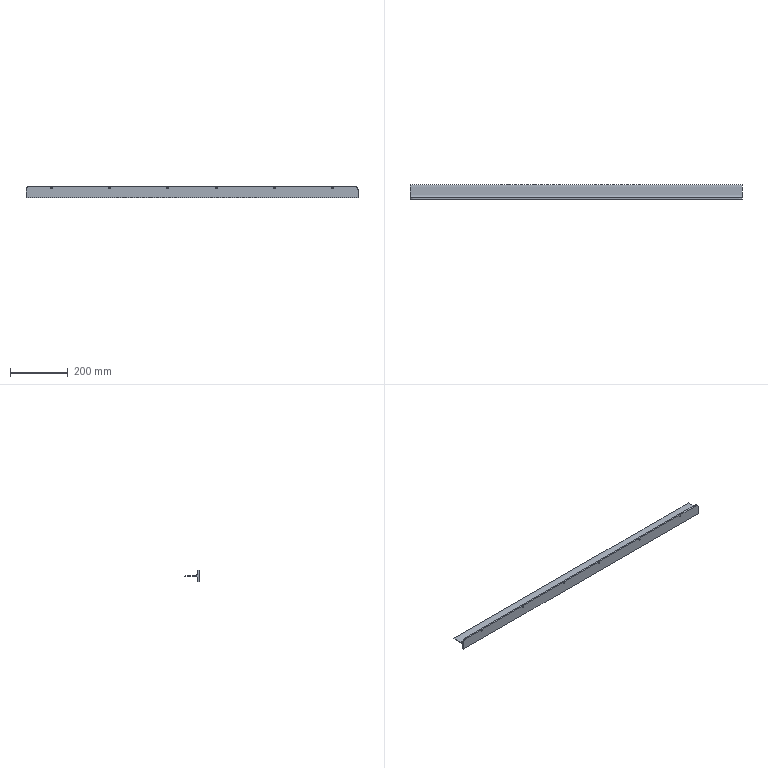Part | NX | features BREP 1 | 1 solid | 25 faces | box 1146 x 50 x 39 mm | volume 357645 mm3 | cylinder 16 | plane 7 | spline 2 | commonest cylinder face diameters 5 x12 20 x2 24 x2
STEP:
#1=CARTESIAN_POINT('',(1058.,-1.616,17.));
#2=VERTEX_POINT('',#1);
#3=CARTESIAN_POINT('',(1058.,-1.616,12.));
#4=VERTEX_POINT('',#3);
#5=CARTESIAN_POINT('',(1058.,-1.616,14.5));
#6=DIRECTION('',(0.,-1.,0.));
#7=DIRECTION('',(0.,0.,1.));
#8=AXIS2_PLACEMENT_3D('',#5,#6,#7);
#9=CIRCLE('',#8,2.5);
#10=EDGE_CURVE('',#2,#4,#9,.T.);
#11=ORIENTED_EDGE('',*,*,#10,.T.);
#12=CARTESIAN_POINT('',(1058.,3.384,12.));
#13=VERTEX_POINT('',#12);
#14=CARTESIAN_POINT('',(1058.,-1.617,12.));
#15=DIRECTION('',(0.,1.,0.));
#16=VECTOR('',#15,1000.);
#17=LINE('',#14,#16);
#18=EDGE_CURVE('',#4,#13,#17,.T.);
#19=ORIENTED_EDGE('',*,*,#18,.T.);
#20=CARTESIAN_POINT('',(1058.,3.384,17.));
#21=VERTEX_POINT('',#20);
#22=CARTESIAN_POINT('',(1058.,3.384,14.5));
#23=DIRECTION('',(0.,1.,0.));
#24=DIRECTION('',(0.,0.,-1.));
#25=AXIS2_PLACEMENT_3D('',#22,#23,#24);
#26=CIRCLE('',#25,2.5);
#27=EDGE_CURVE('',#13,#21,#26,.T.);
#28=ORIENTED_EDGE('',*,*,#27,.T.);
#29=CARTESIAN_POINT('',(1058.,-1.617,17.));
#30=DIRECTION('',(0.,1.,0.));
#31=VECTOR('',#30,1000.);
#32=LINE('',#29,#31);
#33=EDGE_CURVE('',#2,#21,#32,.T.);
#34=ORIENTED_EDGE('',*,*,#33,.F.);
#35=EDGE_LOOP('',(#11,#19,#28,#34));
#36=FACE_BOUND('',#35,.T.);
#37=CARTESIAN_POINT('',(1058.,-1.617,14.5));
#38=DIRECTION('',(0.,1.,0.));
#39=DIRECTION('',(0.,0.,-1.));
#40=AXIS2_PLACEMENT_3D('',#37,#38,#39);
#41=CYLINDRICAL_SURFACE('',#40,2.5);
#42=ADVANCED_FACE('',(#36),#41,.F.);
#43=CARTESIAN_POINT('',(858.,-1.616,17.));
#44=VERTEX_POINT('',#43);
#45=CARTESIAN_POINT('',(858.,-1.616,12.));
#46=VERTEX_POINT('',#45);
#47=CARTESIAN_POINT('',(858.,-1.616,14.5));
#48=DIRECTION('',(0.,-1.,0.));
#49=DIRECTION('',(0.,0.,1.));
#50=AXIS2_PLACEMENT_3D('',#47,#48,#49);
#51=CIRCLE('',#50,2.5);
#52=EDGE_CURVE('',#44,#46,#51,.T.);
#53=ORIENTED_EDGE('',*,*,#52,.T.);
#54=CARTESIAN_POINT('',(858.,3.384,12.));
#55=VERTEX_POINT('',#54);
#56=CARTESIAN_POINT('',(858.,-1.617,12.));
#57=DIRECTION('',(0.,1.,0.));
#58=VECTOR('',#57,1000.);
#59=LINE('',#56,#58);
#60=EDGE_CURVE('',#46,#55,#59,.T.);
#61=ORIENTED_EDGE('',*,*,#60,.T.);
#62=CARTESIAN_POINT('',(858.,3.384,17.));
#63=VERTEX_POINT('',#62);
#64=CARTESIAN_POINT('',(858.,3.384,14.5));
#65=DIRECTION('',(0.,1.,0.));
#66=DIRECTION('',(0.,0.,-1.));
#67=AXIS2_PLACEMENT_3D('',#64,#65,#66);
#68=CIRCLE('',#67,2.5);
#69=EDGE_CURVE('',#55,#63,#68,.T.);
#70=ORIENTED_EDGE('',*,*,#69,.T.);
#71=CARTESIAN_POINT('',(858.,-1.617,17.));
#72=DIRECTION('',(0.,1.,0.));
#73=VECTOR('',#72,1000.);
#74=LINE('',#71,#73);
#75=EDGE_CURVE('',#44,#63,#74,.T.);
#76=ORIENTED_EDGE('',*,*,#75,.F.);
#77=EDGE_LOOP('',(#53,#61,#70,#76));
#78=FACE_BOUND('',#77,.T.);
#79=CARTESIAN_POINT('',(858.,-1.617,14.5));
#80=DIRECTION('',(0.,1.,0.));
#81=DIRECTION('',(0.,0.,-1.));
#82=AXIS2_PLACEMENT_3D('',#79,#80,#81);
#83=CYLINDRICAL_SURFACE('',#82,2.5);
#84=ADVANCED_FACE('',(#78),#83,.F.);
#85=CARTESIAN_POINT('',(88.,-1.616,17.));
#86=VERTEX_POINT('',#85);
#87=CARTESIAN_POINT('',(88.,-1.616,12.));
#88=VERTEX_POINT('',#87);
#89=CARTESIAN_POINT('',(88.,-1.616,14.5));
#90=DIRECTION('',(0.,-1.,0.));
#91=DIRECTION('',(0.,0.,1.));
#92=AXIS2_PLACEMENT_3D('',#89,#90,#91);
#93=CIRCLE('',#92,2.5);
#94=EDGE_CURVE('',#86,#88,#93,.T.);
#95=ORIENTED_EDGE('',*,*,#94,.T.);
#96=CARTESIAN_POINT('',(88.,3.384,12.));
#97=VERTEX_POINT('',#96);
#98=CARTESIAN_POINT('',(88.,-1.617,12.));
#99=DIRECTION('',(0.,1.,0.));
#100=VECTOR('',#99,1000.);
#101=LINE('',#98,#100);
#102=EDGE_CURVE('',#88,#97,#101,.T.);
#103=ORIENTED_EDGE('',*,*,#102,.T.);
#104=CARTESIAN_POINT('',(88.,3.384,17.));
#105=VERTEX_POINT('',#104);
#106=CARTESIAN_POINT('',(88.,3.384,14.5));
#107=DIRECTION('',(0.,1.,0.));
#108=DIRECTION('',(0.,0.,1.));
#109=AXIS2_PLACEMENT_3D('',#106,#107,#108);
#110=CIRCLE('',#109,2.5);
#111=EDGE_CURVE('',#97,#105,#110,.T.);
#112=ORIENTED_EDGE('',*,*,#111,.T.);
#113=CARTESIAN_POINT('',(88.,-1.617,17.));
#114=DIRECTION('',(0.,1.,0.));
#115=VECTOR('',#114,1000.);
#116=LINE('',#113,#115);
#117=EDGE_CURVE('',#86,#105,#116,.T.);
#118=ORIENTED_EDGE('',*,*,#117,.F.);
#119=EDGE_LOOP('',(#95,#103,#112,#118));
#120=FACE_BOUND('',#119,.T.);
#121=CARTESIAN_POINT('',(88.,-1.617,14.5));
#122=DIRECTION('',(0.,1.,0.));
#123=DIRECTION('',(0.,0.,-1.));
#124=AXIS2_PLACEMENT_3D('',#121,#122,#123);
#125=CYLINDRICAL_SURFACE('',#124,2.5);
#126=ADVANCED_FACE('',(#120),#125,.F.);
#127=CARTESIAN_POINT('',(288.,-1.616,17.));
#128=VERTEX_POINT('',#127);
#129=CARTESIAN_POINT('',(288.,-1.616,12.));
#130=VERTEX_POINT('',#129);
#131=CARTESIAN_POINT('',(288.,-1.616,14.5));
#132=DIRECTION('',(0.,-1.,0.));
#133=DIRECTION('',(0.,0.,1.));
#134=AXIS2_PLACEMENT_3D('',#131,#132,#133);
#135=CIRCLE('',#134,2.5);
#136=EDGE_CURVE('',#128,#130,#135,.T.);
#137=ORIENTED_EDGE('',*,*,#136,.T.);
#138=CARTESIAN_POINT('',(288.,3.384,12.));
#139=VERTEX_POINT('',#138);
#140=CARTESIAN_POINT('',(288.,-1.617,12.));
#141=DIRECTION('',(0.,1.,0.));
#142=VECTOR('',#141,1000.);
#143=LINE('',#140,#142);
#144=EDGE_CURVE('',#130,#139,#143,.T.);
#145=ORIENTED_EDGE('',*,*,#144,.T.);
#146=CARTESIAN_POINT('',(288.,3.384,17.));
#147=VERTEX_POINT('',#146);
#148=CARTESIAN_POINT('',(288.,3.384,14.5));
#149=DIRECTION('',(0.,1.,0.));
#150=DIRECTION('',(0.,0.,1.));
#151=AXIS2_PLACEMENT_3D('',#148,#149,#150);
#152=CIRCLE('',#151,2.5);
#153=EDGE_CURVE('',#139,#147,#152,.T.);
#154=ORIENTED_EDGE('',*,*,#153,.T.);
#155=CARTESIAN_POINT('',(288.,-1.617,17.));
#156=DIRECTION('',(0.,1.,0.));
#157=VECTOR('',#156,1000.);
#158=LINE('',#155,#157);
#159=EDGE_CURVE('',#128,#147,#158,.T.);
#160=ORIENTED_EDGE('',*,*,#159,.F.);
#161=EDGE_LOOP('',(#137,#145,#154,#160));
#162=FACE_BOUND('',#161,.T.);
#163=CARTESIAN_POINT('',(288.,-1.617,14.5));
#164=DIRECTION('',(0.,1.,0.));
#165=DIRECTION('',(0.,0.,-1.));
#166=AXIS2_PLACEMENT_3D('',#163,#164,#165);
#167=CYLINDRICAL_SURFACE('',#166,2.5);
#168=ADVANCED_FACE('',(#162),#167,.F.);
#169=CARTESIAN_POINT('',(658.,-1.616,17.));
#170=VERTEX_POINT('',#169);
#171=CARTESIAN_POINT('',(658.,-1.616,12.));
#172=VERTEX_POINT('',#171);
#173=CARTESIAN_POINT('',(658.,-1.616,14.5));
#174=DIRECTION('',(0.,-1.,0.));
#175=DIRECTION('',(0.,0.,1.));
#176=AXIS2_PLACEMENT_3D('',#173,#174,#175);
#177=CIRCLE('',#176,2.5);
#178=EDGE_CURVE('',#170,#172,#177,.T.);
#179=ORIENTED_EDGE('',*,*,#178,.T.);
#180=CARTESIAN_POINT('',(658.,3.384,12.));
#181=VERTEX_POINT('',#180);
#182=CARTESIAN_POINT('',(658.,-1.617,12.));
#183=DIRECTION('',(0.,1.,0.));
#184=VECTOR('',#183,1000.);
#185=LINE('',#182,#184);
#186=EDGE_CURVE('',#172,#181,#185,.T.);
#187=ORIENTED_EDGE('',*,*,#186,.T.);
#188=CARTESIAN_POINT('',(658.,3.384,17.));
#189=VERTEX_POINT('',#188);
#190=CARTESIAN_POINT('',(658.,3.384,14.5));
#191=DIRECTION('',(0.,1.,0.));
#192=DIRECTION('',(0.,0.,-1.));
#193=AXIS2_PLACEMENT_3D('',#190,#191,#192);
#194=CIRCLE('',#193,2.5);
#195=EDGE_CURVE('',#181,#189,#194,.T.);
#196=ORIENTED_EDGE('',*,*,#195,.T.);
#197=CARTESIAN_POINT('',(658.,-1.617,17.));
#198=DIRECTION('',(0.,1.,0.));
#199=VECTOR('',#198,1000.);
#200=LINE('',#197,#199);
#201=EDGE_CURVE('',#170,#189,#200,.T.);
#202=ORIENTED_EDGE('',*,*,#201,.F.);
#203=EDGE_LOOP('',(#179,#187,#196,#202));
#204=FACE_BOUND('',#203,.T.);
#205=CARTESIAN_POINT('',(658.,-1.617,14.5));
#206=DIRECTION('',(0.,1.,0.));
#207=DIRECTION('',(0.,0.,-1.));
#208=AXIS2_PLACEMENT_3D('',#205,#206,#207);
#209=CYLINDRICAL_SURFACE('',#208,2.5);
#210=ADVANCED_FACE('',(#204),#209,.F.);
#211=CARTESIAN_POINT('',(488.,-1.616,17.));
#212=VERTEX_POINT('',#211);
#213=CARTESIAN_POINT('',(488.,-1.616,12.));
#214=VERTEX_POINT('',#213);
#215=CARTESIAN_POINT('',(488.,-1.616,14.5));
#216=DIRECTION('',(0.,-1.,0.));
#217=DIRECTION('',(0.,0.,1.));
#218=AXIS2_PLACEMENT_3D('',#215,#216,#217);
#219=CIRCLE('',#218,2.5);
#220=EDGE_CURVE('',#212,#214,#219,.T.);
#221=ORIENTED_EDGE('',*,*,#220,.T.);
#222=CARTESIAN_POINT('',(488.,3.384,12.));
#223=VERTEX_POINT('',#222);
#224=CARTESIAN_POINT('',(488.,-1.617,12.));
#225=DIRECTION('',(0.,1.,0.));
#226=VECTOR('',#225,1000.);
#227=LINE('',#224,#226);
#228=EDGE_CURVE('',#214,#223,#227,.T.);
#229=ORIENTED_EDGE('',*,*,#228,.T.);
#230=CARTESIAN_POINT('',(488.,3.384,17.));
#231=VERTEX_POINT('',#230);
#232=CARTESIAN_POINT('',(488.,3.384,14.5));
#233=DIRECTION('',(0.,1.,0.));
#234=DIRECTION('',(0.,0.,1.));
#235=AXIS2_PLACEMENT_3D('',#232,#233,#234);
#236=CIRCLE('',#235,2.5);
#237=EDGE_CURVE('',#223,#231,#236,.T.);
#238=ORIENTED_EDGE('',*,*,#237,.T.);
#239=CARTESIAN_POINT('',(488.,-1.617,17.));
#240=DIRECTION('',(0.,1.,0.));
#241=VECTOR('',#240,1000.);
#242=LINE('',#239,#241);
#243=EDGE_CURVE('',#212,#231,#242,.T.);
#244=ORIENTED_EDGE('',*,*,#243,.F.);
#245=EDGE_LOOP('',(#221,#229,#238,#244));
#246=FACE_BOUND('',#245,.T.);
#247=CARTESIAN_POINT('',(488.,-1.617,14.5));
#248=DIRECTION('',(0.,1.,0.));
#249=DIRECTION('',(0.,0.,-1.));
#250=AXIS2_PLACEMENT_3D('',#247,#248,#249);
#251=CYLINDRICAL_SURFACE('',#250,2.5);
#252=ADVANCED_FACE('',(#246),#251,.F.);
#253=CARTESIAN_POINT('',(1134.,-1.616,19.5));
#254=VERTEX_POINT('',#253);
#255=CARTESIAN_POINT('',(12.,-1.616,19.5));
#256=VERTEX_POINT('',#255);
#257=CARTESIAN_POINT('',(1146.,-1.616,19.5));
#258=DIRECTION('',(-1.,0.,0.));
#259=VECTOR('',#258,1000.);
#260=LINE('',#257,#259);
#261=EDGE_CURVE('',#254,#256,#260,.T.);
#262=ORIENTED_EDGE('',*,*,#261,.F.);
#263=CARTESIAN_POINT('',(1134.,3.384,19.5));
#264=VERTEX_POINT('',#263);
#265=CARTESIAN_POINT('',(1134.,48.385,19.5));
#266=DIRECTION('',(0.,-1.,0.));
#267=VECTOR('',#266,1000.);
#268=LINE('',#265,#267);
#269=EDGE_CURVE('',#264,#254,#268,.T.);
#270=ORIENTED_EDGE('',*,*,#269,.F.);
#271=CARTESIAN_POINT('',(12.,3.384,19.5));
#272=VERTEX_POINT('',#271);
#273=CARTESIAN_POINT('',(1146.,3.384,19.5));
#274=DIRECTION('',(-1.,0.,0.));
#275=VECTOR('',#274,1000.);
#276=LINE('',#273,#275);
#277=EDGE_CURVE('',#264,#272,#276,.T.);
#278=ORIENTED_EDGE('',*,*,#277,.T.);
#279=CARTESIAN_POINT('',(12.,48.385,19.5));
#280=DIRECTION('',(0.,-1.,0.));
#281=VECTOR('',#280,1000.);
#282=LINE('',#279,#281);
#283=EDGE_CURVE('',#272,#256,#282,.T.);
#284=ORIENTED_EDGE('',*,*,#283,.T.);
#285=EDGE_LOOP('',(#262,#270,#278,#284));
#286=FACE_BOUND('',#285,.T.);
#287=CARTESIAN_POINT('',(1146.,3.384,19.5));
#288=DIRECTION('',(0.,0.,-1.));
#289=DIRECTION('',(0.,1.,0.));
#290=AXIS2_PLACEMENT_3D('',#287,#288,#289);
#291=PLANE('',#290);
#292=ADVANCED_FACE('',(#286),#291,.F.);
#293=CARTESIAN_POINT('',(0.,-1.616,-19.5));
#294=VERTEX_POINT('',#293);
#295=CARTESIAN_POINT('',(0.,3.384,-19.5));
#296=VERTEX_POINT('',#295);
#297=CARTESIAN_POINT('',(0.,3.384,-19.5));
#298=DIRECTION('',(0.,1.,0.));
#299=VECTOR('',#298,1000.);
#300=LINE('',#297,#299);
#301=EDGE_CURVE('',#294,#296,#300,.T.);
#302=ORIENTED_EDGE('',*,*,#301,.T.);
#303=CARTESIAN_POINT('',(1146.,3.384,-19.5));
#304=VERTEX_POINT('',#303);
#305=CARTESIAN_POINT('',(1146.,3.384,-19.5));
#306=DIRECTION('',(-1.,0.,0.));
#307=VECTOR('',#306,1000.);
#308=LINE('',#305,#307);
#309=EDGE_CURVE('',#304,#296,#308,.T.);
#310=ORIENTED_EDGE('',*,*,#309,.F.);
#311=CARTESIAN_POINT('',(1146.,-1.616,-19.5));
#312=VERTEX_POINT('',#311);
#313=CARTESIAN_POINT('',(1146.,3.384,-19.5));
#314=DIRECTION('',(0.,1.,0.));
#315=VECTOR('',#314,1000.);
#316=LINE('',#313,#315);
#317=EDGE_CURVE('',#312,#304,#316,.T.);
#318=ORIENTED_EDGE('',*,*,#317,.F.);
#319=CARTESIAN_POINT('',(1146.,-1.616,-19.5));
#320=DIRECTION('',(-1.,0.,0.));
#321=VECTOR('',#320,1000.);
#322=LINE('',#319,#321);
#323=EDGE_CURVE('',#312,#294,#322,.T.);
#324=ORIENTED_EDGE('',*,*,#323,.T.);
#325=EDGE_LOOP('',(#302,#310,#318,#324));
#326=FACE_BOUND('',#325,.T.);
#327=CARTESIAN_POINT('',(1146.,3.384,-19.5));
#328=DIRECTION('',(0.,0.,1.));
#329=DIRECTION('',(0.,1.,0.));
#330=AXIS2_PLACEMENT_3D('',#327,#328,#329);
#331=PLANE('',#330);
#332=ADVANCED_FACE('',(#326),#331,.F.);
#333=CARTESIAN_POINT('',(0.,3.384,-10.913));
#334=VERTEX_POINT('',#333);
#335=CARTESIAN_POINT('',(0.,3.384,-10.913));
#336=DIRECTION('',(0.,0.,1.));
#337=VECTOR('',#336,1000.);
#338=LINE('',#335,#337);
#339=EDGE_CURVE('',#296,#334,#338,.T.);
#340=ORIENTED_EDGE('',*,*,#339,.T.);
#341=CARTESIAN_POINT('',(1146.,3.384,-10.913));
#342=VERTEX_POINT('',#341);
#343=CARTESIAN_POINT('',(1146.,3.384,-10.913));
#344=DIRECTION('',(-1.,0.,0.));
#345=VECTOR('',#344,1000.);
#346=LINE('',#343,#345);
#347=EDGE_CURVE('',#342,#334,#346,.T.);
#348=ORIENTED_EDGE('',*,*,#347,.F.);
#349=CARTESIAN_POINT('',(1146.,3.384,-10.913));
#350=DIRECTION('',(0.,0.,1.));
#351=VECTOR('',#350,1000.);
#352=LINE('',#349,#351);
#353=EDGE_CURVE('',#304,#342,#352,.T.);
#354=ORIENTED_EDGE('',*,*,#353,.F.);
#355=ORIENTED_EDGE('',*,*,#309,.T.);
#356=EDGE_LOOP('',(#340,#348,#354,#355));
#357=FACE_BOUND('',#356,.T.);
#358=CARTESIAN_POINT('',(1146.,3.384,-10.913));
#359=DIRECTION('',(0.,-1.,0.));
#360=DIRECTION('',(1.,0.,0.));
#361=AXIS2_PLACEMENT_3D('',#358,#359,#360);
#362=PLANE('',#361);
#363=ADVANCED_FACE('',(#357),#362,.F.);
#364=CARTESIAN_POINT('',(0.,12.421,-0.9595));
#365=VERTEX_POINT('',#364);
#366=CARTESIAN_POINT('',(0.,13.384,-10.913));
#367=DIRECTION('',(-1.,0.,0.));
#368=DIRECTION('',(0.,0.,1.));
#369=AXIS2_PLACEMENT_3D('',#366,#367,#368);
#370=CIRCLE('',#369,10.);
#371=EDGE_CURVE('',#334,#365,#370,.T.);
#372=ORIENTED_EDGE('',*,*,#371,.T.);
#373=CARTESIAN_POINT('',(1146.,12.421,-0.9595));
#374=VERTEX_POINT('',#373);
#375=CARTESIAN_POINT('',(1146.,12.421,-0.9595));
#376=DIRECTION('',(-1.,0.,0.));
#377=VECTOR('',#376,1000.);
#378=LINE('',#375,#377);
#379=EDGE_CURVE('',#374,#365,#378,.T.);
#380=ORIENTED_EDGE('',*,*,#379,.F.);
#381=CARTESIAN_POINT('',(1146.,13.384,-10.913));
#382=DIRECTION('',(-1.,0.,0.));
#383=DIRECTION('',(0.,0.,1.));
#384=AXIS2_PLACEMENT_3D('',#381,#382,#383);
#385=CIRCLE('',#384,10.);
#386=EDGE_CURVE('',#342,#374,#385,.T.);
#387=ORIENTED_EDGE('',*,*,#386,.F.);
#388=ORIENTED_EDGE('',*,*,#347,.T.);
#389=EDGE_LOOP('',(#372,#380,#387,#388));
#390=FACE_BOUND('',#389,.T.);
#391=CARTESIAN_POINT('',(1146.,13.384,-10.913));
#392=DIRECTION('',(-1.,0.,0.));
#393=DIRECTION('',(0.,0.,-1.));
#394=AXIS2_PLACEMENT_3D('',#391,#392,#393);
#395=CYLINDRICAL_SURFACE('',#394,10.);
#396=ADVANCED_FACE('',(#390),#395,.F.);
#397=CARTESIAN_POINT('',(0.,48.384,0.));
#398=VERTEX_POINT('',#397);
#399=CARTESIAN_POINT('',(0.,12.421,-0.9595));
#400=CARTESIAN_POINT('',(0.,24.315,0.1902));
#401=CARTESIAN_POINT('',(0.,36.646,-2.478));
#402=CARTESIAN_POINT('',(0.,48.384,0.));
#403=B_SPLINE_CURVE_WITH_KNOTS('',3,(#399,#400,#401,#402),.UNSPECIFIED.,.F.,.F.,(4,4),(0.,1.),.PIECEWISE_BEZIER_KNOTS.);
#404=EDGE_CURVE('',#365,#398,#403,.T.);
#405=ORIENTED_EDGE('',*,*,#404,.T.);
#406=CARTESIAN_POINT('',(1146.,48.384,0.));
#407=VERTEX_POINT('',#406);
#408=CARTESIAN_POINT('',(1146.,48.384,0.));
#409=DIRECTION('',(-1.,0.,0.));
#410=VECTOR('',#409,1000.);
#411=LINE('',#408,#410);
#412=EDGE_CURVE('',#407,#398,#411,.T.);
#413=ORIENTED_EDGE('',*,*,#412,.F.);
#414=CARTESIAN_POINT('',(1146.,12.421,-0.9595));
#415=CARTESIAN_POINT('',(1146.,24.315,0.1902));
#416=CARTESIAN_POINT('',(1146.,36.646,-2.478));
#417=CARTESIAN_POINT('',(1146.,48.384,0.));
#418=B_SPLINE_CURVE_WITH_KNOTS('',3,(#414,#415,#416,#417),.UNSPECIFIED.,.F.,.F.,(4,4),(0.,1.),.PIECEWISE_BEZIER_KNOTS.);
#419=EDGE_CURVE('',#374,#407,#418,.T.);
#420=ORIENTED_EDGE('',*,*,#419,.F.);
#421=ORIENTED_EDGE('',*,*,#379,.T.);
#422=EDGE_LOOP('',(#405,#413,#420,#421));
#423=FACE_BOUND('',#422,.T.);
#424=CARTESIAN_POINT('',(1146.,12.421,-0.9595));
#425=CARTESIAN_POINT('',(0.,12.421,-0.9595));
#426=CARTESIAN_POINT('',(1146.,24.315,0.1902));
#427=CARTESIAN_POINT('',(0.,24.315,0.1902));
#428=CARTESIAN_POINT('',(1146.,36.646,-2.478));
#429=CARTESIAN_POINT('',(0.,36.646,-2.478));
#430=CARTESIAN_POINT('',(1146.,48.384,0.));
#431=CARTESIAN_POINT('',(0.,48.384,0.));
#432=B_SPLINE_SURFACE_WITH_KNOTS('',3,1,((#424,#425),(#426,#427),(#428,#429),(#430,#431)),.SURF_OF_LINEAR_EXTRUSION.,.F.,.F.,.F.,(4,4),(2,2),(0.,1.),(0.,1.),.PIECEWISE_BEZIER_KNOTS.);
#433=ADVANCED_FACE('',(#423),#432,.F.);
#434=CARTESIAN_POINT('',(0.,12.421,0.9595));
#435=VERTEX_POINT('',#434);
#436=CARTESIAN_POINT('',(0.,48.384,0.));
#437=CARTESIAN_POINT('',(0.,36.646,2.478));
#438=CARTESIAN_POINT('',(0.,24.315,-0.1902));
#439=CARTESIAN_POINT('',(0.,12.421,0.9595));
#440=B_SPLINE_CURVE_WITH_KNOTS('',3,(#436,#437,#438,#439),.UNSPECIFIED.,.F.,.F.,(4,4),(0.,1.),.PIECEWISE_BEZIER_KNOTS.);
#441=EDGE_CURVE('',#398,#435,#440,.T.);
#442=ORIENTED_EDGE('',*,*,#441,.T.);
#443=CARTESIAN_POINT('',(1146.,12.421,0.9595));
#444=VERTEX_POINT('',#443);
#445=CARTESIAN_POINT('',(1146.,12.421,0.9595));
#446=DIRECTION('',(-1.,0.,0.));
#447=VECTOR('',#446,1000.);
#448=LINE('',#445,#447);
#449=EDGE_CURVE('',#444,#435,#448,.T.);
#450=ORIENTED_EDGE('',*,*,#449,.F.);
#451=CARTESIAN_POINT('',(1146.,48.384,0.));
#452=CARTESIAN_POINT('',(1146.,36.646,2.478));
#453=CARTESIAN_POINT('',(1146.,24.315,-0.1902));
#454=CARTESIAN_POINT('',(1146.,12.421,0.9595));
#455=B_SPLINE_CURVE_WITH_KNOTS('',3,(#451,#452,#453,#454),.UNSPECIFIED.,.F.,.F.,(4,4),(0.,1.),.PIECEWISE_BEZIER_KNOTS.);
#456=EDGE_CURVE('',#407,#444,#455,.T.);
#457=ORIENTED_EDGE('',*,*,#456,.F.);
#458=ORIENTED_EDGE('',*,*,#412,.T.);
#459=EDGE_LOOP('',(#442,#450,#457,#458));
#460=FACE_BOUND('',#459,.T.);
#461=CARTESIAN_POINT('',(1146.,48.384,0.));
#462=CARTESIAN_POINT('',(0.,48.384,0.));
#463=CARTESIAN_POINT('',(1146.,36.646,2.478));
#464=CARTESIAN_POINT('',(0.,36.646,2.478));
#465=CARTESIAN_POINT('',(1146.,24.315,-0.1902));
#466=CARTESIAN_POINT('',(0.,24.315,-0.1902));
#467=CARTESIAN_POINT('',(1146.,12.421,0.9595));
#468=CARTESIAN_POINT('',(0.,12.421,0.9595));
#469=B_SPLINE_SURFACE_WITH_KNOTS('',3,1,((#461,#462),(#463,#464),(#465,#466),(#467,#468)),.SURF_OF_LINEAR_EXTRUSION.,.F.,.F.,.F.,(4,4),(2,2),(0.,1.),(0.,1.),.PIECEWISE_BEZIER_KNOTS.);
#470=ADVANCED_FACE('',(#460),#469,.F.);
#471=CARTESIAN_POINT('',(1145.504,3.384,10.913));
#472=VERTEX_POINT('',#471);
#473=CARTESIAN_POINT('',(0.4956,3.384,10.913));
#474=VERTEX_POINT('',#473);
#475=CARTESIAN_POINT('',(1146.,3.384,10.913));
#476=DIRECTION('',(-1.,0.,0.));
#477=VECTOR('',#476,1000.);
#478=LINE('',#475,#477);
#479=EDGE_CURVE('',#472,#474,#478,.T.);
#480=ORIENTED_EDGE('',*,*,#479,.F.);
#481=CARTESIAN_POINT('',(1146.,3.984,7.5));
#482=VERTEX_POINT('',#481);
#483=CARTESIAN_POINT('',(1146.,3.984,7.5));
#484=CARTESIAN_POINT('',(1146.,3.579,8.614));
#485=CARTESIAN_POINT('',(1145.842,3.384,9.776));
#486=CARTESIAN_POINT('',(1145.504,3.384,10.913));
#487=B_SPLINE_CURVE_WITH_KNOTS('',3,(#483,#484,#485,#486),.UNSPECIFIED.,.F.,.F.,(4,4),(0.,0.003506),.UNSPECIFIED.);
#488=EDGE_CURVE('',#482,#472,#487,.T.);
#489=ORIENTED_EDGE('',*,*,#488,.F.);
#490=CARTESIAN_POINT('',(1146.,13.384,10.913));
#491=DIRECTION('',(-1.,0.,0.));
#492=DIRECTION('',(0.,0.,-1.));
#493=AXIS2_PLACEMENT_3D('',#490,#491,#492);
#494=CIRCLE('',#493,10.);
#495=EDGE_CURVE('',#444,#482,#494,.T.);
#496=ORIENTED_EDGE('',*,*,#495,.F.);
#497=ORIENTED_EDGE('',*,*,#449,.T.);
#498=CARTESIAN_POINT('',(0.,3.984,7.5));
#499=VERTEX_POINT('',#498);
#500=CARTESIAN_POINT('',(0.,13.384,10.913));
#501=DIRECTION('',(-1.,0.,0.));
#502=DIRECTION('',(0.,0.,-1.));
#503=AXIS2_PLACEMENT_3D('',#500,#501,#502);
#504=CIRCLE('',#503,10.);
#505=EDGE_CURVE('',#435,#499,#504,.T.);
#506=ORIENTED_EDGE('',*,*,#505,.T.);
#507=CARTESIAN_POINT('',(0.4956,3.384,10.913));
#508=CARTESIAN_POINT('',(0.1584,3.384,9.777));
#509=CARTESIAN_POINT('',(0.,3.579,8.615));
#510=CARTESIAN_POINT('',(0.,3.984,7.5));
#511=B_SPLINE_CURVE_WITH_KNOTS('',3,(#507,#508,#509,#510),.UNSPECIFIED.,.F.,.F.,(4,4),(0.,0.003506),.UNSPECIFIED.);
#512=EDGE_CURVE('',#474,#499,#511,.T.);
#513=ORIENTED_EDGE('',*,*,#512,.F.);
#514=EDGE_LOOP('',(#480,#489,#496,#497,#506,#513));
#515=FACE_BOUND('',#514,.T.);
#516=CARTESIAN_POINT('',(1146.,13.384,10.913));
#517=DIRECTION('',(-1.,0.,0.));
#518=DIRECTION('',(0.,0.,-1.));
#519=AXIS2_PLACEMENT_3D('',#516,#517,#518);
#520=CYLINDRICAL_SURFACE('',#519,10.);
#521=ADVANCED_FACE('',(#515),#520,.F.);
#522=ORIENTED_EDGE('',*,*,#277,.F.);
#523=CARTESIAN_POINT('',(1134.,3.384,7.5));
#524=DIRECTION('',(0.,-1.,0.));
#525=DIRECTION('',(0.,0.,-1.));
#526=AXIS2_PLACEMENT_3D('',#523,#524,#525);
#527=CIRCLE('',#526,12.);
#528=EDGE_CURVE('',#472,#264,#527,.T.);
#529=ORIENTED_EDGE('',*,*,#528,.F.);
#530=ORIENTED_EDGE('',*,*,#479,.T.);
#531=CARTESIAN_POINT('',(12.,3.384,7.5));
#532=DIRECTION('',(0.,-1.,0.));
#533=DIRECTION('',(0.,0.,-1.));
#534=AXIS2_PLACEMENT_3D('',#531,#532,#533);
#535=CIRCLE('',#534,12.);
#536=EDGE_CURVE('',#272,#474,#535,.T.);
#537=ORIENTED_EDGE('',*,*,#536,.F.);
#538=EDGE_LOOP('',(#522,#529,#530,#537));
#539=FACE_BOUND('',#538,.T.);
#540=CARTESIAN_POINT('',(1058.,3.384,14.5));
#541=DIRECTION('',(0.,1.,0.));
#542=DIRECTION('',(0.,0.,-1.));
#543=AXIS2_PLACEMENT_3D('',#540,#541,#542);
#544=CIRCLE('',#543,2.5);
#545=EDGE_CURVE('',#21,#13,#544,.T.);
#546=ORIENTED_EDGE('',*,*,#545,.F.);
#547=ORIENTED_EDGE('',*,*,#27,.F.);
#548=EDGE_LOOP('',(#546,#547));
#549=FACE_BOUND('',#548,.T.);
#550=CARTESIAN_POINT('',(858.,3.384,14.5));
#551=DIRECTION('',(0.,1.,0.));
#552=DIRECTION('',(0.,0.,-1.));
#553=AXIS2_PLACEMENT_3D('',#550,#551,#552);
#554=CIRCLE('',#553,2.5);
#555=EDGE_CURVE('',#63,#55,#554,.T.);
#556=ORIENTED_EDGE('',*,*,#555,.F.);
#557=ORIENTED_EDGE('',*,*,#69,.F.);
#558=EDGE_LOOP('',(#556,#557));
#559=FACE_BOUND('',#558,.T.);
#560=CARTESIAN_POINT('',(88.,3.384,14.5));
#561=DIRECTION('',(0.,1.,0.));
#562=DIRECTION('',(0.,0.,1.));
#563=AXIS2_PLACEMENT_3D('',#560,#561,#562);
#564=CIRCLE('',#563,2.5);
#565=EDGE_CURVE('',#105,#97,#564,.T.);
#566=ORIENTED_EDGE('',*,*,#565,.F.);
#567=ORIENTED_EDGE('',*,*,#111,.F.);
#568=EDGE_LOOP('',(#566,#567));
#569=FACE_BOUND('',#568,.T.);
#570=CARTESIAN_POINT('',(288.,3.384,14.5));
#571=DIRECTION('',(0.,1.,0.));
#572=DIRECTION('',(0.,0.,1.));
#573=AXIS2_PLACEMENT_3D('',#570,#571,#572);
#574=CIRCLE('',#573,2.5);
#575=EDGE_CURVE('',#147,#139,#574,.T.);
#576=ORIENTED_EDGE('',*,*,#575,.F.);
#577=ORIENTED_EDGE('',*,*,#153,.F.);
#578=EDGE_LOOP('',(#576,#577));
#579=FACE_BOUND('',#578,.T.);
#580=CARTESIAN_POINT('',(658.,3.384,14.5));
#581=DIRECTION('',(0.,1.,0.));
#582=DIRECTION('',(0.,0.,-1.));
#583=AXIS2_PLACEMENT_3D('',#580,#581,#582);
#584=CIRCLE('',#583,2.5);
#585=EDGE_CURVE('',#189,#181,#584,.T.);
#586=ORIENTED_EDGE('',*,*,#585,.F.);
#587=ORIENTED_EDGE('',*,*,#195,.F.);
#588=EDGE_LOOP('',(#586,#587));
#589=FACE_BOUND('',#588,.T.);
#590=CARTESIAN_POINT('',(488.,3.384,14.5));
#591=DIRECTION('',(0.,1.,0.));
#592=DIRECTION('',(0.,0.,1.));
#593=AXIS2_PLACEMENT_3D('',#590,#591,#592);
#594=CIRCLE('',#593,2.5);
#595=EDGE_CURVE('',#231,#223,#594,.T.);
#596=ORIENTED_EDGE('',*,*,#595,.F.);
#597=ORIENTED_EDGE('',*,*,#237,.F.);
#598=EDGE_LOOP('',(#596,#597));
#599=FACE_BOUND('',#598,.T.);
#600=CARTESIAN_POINT('',(1146.,3.384,19.5));
#601=DIRECTION('',(0.,-1.,0.));
#602=DIRECTION('',(1.,0.,0.));
#603=AXIS2_PLACEMENT_3D('',#600,#601,#602);
#604=PLANE('',#603);
#605=ADVANCED_FACE('',(#539,#549,#559,#569,#579,#589,#599),#604,.F.);
#606=CARTESIAN_POINT('',(1146.,-1.616,7.5));
#607=VERTEX_POINT('',#606);
#608=CARTESIAN_POINT('',(1146.,-1.616,19.5));
#609=DIRECTION('',(0.,0.,-1.));
#610=VECTOR('',#609,1000.);
#611=LINE('',#608,#610);
#612=EDGE_CURVE('',#607,#312,#611,.T.);
#613=ORIENTED_EDGE('',*,*,#612,.F.);
#614=CARTESIAN_POINT('',(1134.,-1.616,7.5));
#615=DIRECTION('',(0.,1.,0.));
#616=DIRECTION('',(0.,0.,1.));
#617=AXIS2_PLACEMENT_3D('',#614,#615,#616);
#618=CIRCLE('',#617,12.);
#619=EDGE_CURVE('',#254,#607,#618,.T.);
#620=ORIENTED_EDGE('',*,*,#619,.F.);
#621=ORIENTED_EDGE('',*,*,#261,.T.);
#622=CARTESIAN_POINT('',(0.,-1.616,7.5));
#623=VERTEX_POINT('',#622);
#624=CARTESIAN_POINT('',(12.,-1.616,7.5));
#625=DIRECTION('',(0.,1.,0.));
#626=DIRECTION('',(0.,0.,-1.));
#627=AXIS2_PLACEMENT_3D('',#624,#625,#626);
#628=CIRCLE('',#627,12.);
#629=EDGE_CURVE('',#623,#256,#628,.T.);
#630=ORIENTED_EDGE('',*,*,#629,.F.);
#631=CARTESIAN_POINT('',(0.,-1.616,19.5));
#632=DIRECTION('',(0.,0.,-1.));
#633=VECTOR('',#632,1000.);
#634=LINE('',#631,#633);
#635=EDGE_CURVE('',#623,#294,#634,.T.);
#636=ORIENTED_EDGE('',*,*,#635,.T.);
#637=ORIENTED_EDGE('',*,*,#323,.F.);
#638=EDGE_LOOP('',(#613,#620,#621,#630,#636,#637));
#639=FACE_BOUND('',#638,.T.);
#640=ORIENTED_EDGE('',*,*,#10,.F.);
#641=CARTESIAN_POINT('',(1058.,-1.616,14.5));
#642=DIRECTION('',(0.,-1.,0.));
#643=DIRECTION('',(0.,0.,1.));
#644=AXIS2_PLACEMENT_3D('',#641,#642,#643);
#645=CIRCLE('',#644,2.5);
#646=EDGE_CURVE('',#4,#2,#645,.T.);
#647=ORIENTED_EDGE('',*,*,#646,.F.);
#648=EDGE_LOOP('',(#640,#647));
#649=FACE_BOUND('',#648,.T.);
#650=ORIENTED_EDGE('',*,*,#52,.F.);
#651=CARTESIAN_POINT('',(858.,-1.616,14.5));
#652=DIRECTION('',(0.,-1.,0.));
#653=DIRECTION('',(0.,0.,1.));
#654=AXIS2_PLACEMENT_3D('',#651,#652,#653);
#655=CIRCLE('',#654,2.5);
#656=EDGE_CURVE('',#46,#44,#655,.T.);
#657=ORIENTED_EDGE('',*,*,#656,.F.);
#658=EDGE_LOOP('',(#650,#657));
#659=FACE_BOUND('',#658,.T.);
#660=ORIENTED_EDGE('',*,*,#94,.F.);
#661=CARTESIAN_POINT('',(88.,-1.616,14.5));
#662=DIRECTION('',(0.,-1.,0.));
#663=DIRECTION('',(0.,0.,1.));
#664=AXIS2_PLACEMENT_3D('',#661,#662,#663);
#665=CIRCLE('',#664,2.5);
#666=EDGE_CURVE('',#88,#86,#665,.T.);
#667=ORIENTED_EDGE('',*,*,#666,.F.);
#668=EDGE_LOOP('',(#660,#667));
#669=FACE_BOUND('',#668,.T.);
#670=ORIENTED_EDGE('',*,*,#136,.F.);
#671=CARTESIAN_POINT('',(288.,-1.616,14.5));
#672=DIRECTION('',(0.,-1.,0.));
#673=DIRECTION('',(0.,0.,1.));
#674=AXIS2_PLACEMENT_3D('',#671,#672,#673);
#675=CIRCLE('',#674,2.5);
#676=EDGE_CURVE('',#130,#128,#675,.T.);
#677=ORIENTED_EDGE('',*,*,#676,.F.);
#678=EDGE_LOOP('',(#670,#677));
#679=FACE_BOUND('',#678,.T.);
#680=ORIENTED_EDGE('',*,*,#178,.F.);
#681=CARTESIAN_POINT('',(658.,-1.616,14.5));
#682=DIRECTION('',(0.,-1.,0.));
#683=DIRECTION('',(0.,0.,1.));
#684=AXIS2_PLACEMENT_3D('',#681,#682,#683);
#685=CIRCLE('',#684,2.5);
#686=EDGE_CURVE('',#172,#170,#685,.T.);
#687=ORIENTED_EDGE('',*,*,#686,.F.);
#688=EDGE_LOOP('',(#680,#687));
#689=FACE_BOUND('',#688,.T.);
#690=ORIENTED_EDGE('',*,*,#220,.F.);
#691=CARTESIAN_POINT('',(488.,-1.616,14.5));
#692=DIRECTION('',(0.,-1.,0.));
#693=DIRECTION('',(0.,0.,1.));
#694=AXIS2_PLACEMENT_3D('',#691,#692,#693);
#695=CIRCLE('',#694,2.5);
#696=EDGE_CURVE('',#214,#212,#695,.T.);
#697=ORIENTED_EDGE('',*,*,#696,.F.);
#698=EDGE_LOOP('',(#690,#697));
#699=FACE_BOUND('',#698,.T.);
#700=CARTESIAN_POINT('',(1146.,-1.616,19.5));
#701=DIRECTION('',(0.,1.,0.));
#702=DIRECTION('',(0.,0.,1.));
#703=AXIS2_PLACEMENT_3D('',#700,#701,#702);
#704=PLANE('',#703);
#705=ADVANCED_FACE('',(#639,#649,#659,#669,#679,#689,#699),#704,.F.);
#706=CARTESIAN_POINT('',(1146.,48.385,7.5));
#707=DIRECTION('',(0.,-1.,0.));
#708=VECTOR('',#707,1000.);
#709=LINE('',#706,#708);
#710=EDGE_CURVE('',#482,#607,#709,.T.);
#711=ORIENTED_EDGE('',*,*,#710,.T.);
#712=ORIENTED_EDGE('',*,*,#612,.T.);
#713=ORIENTED_EDGE('',*,*,#317,.T.);
#714=ORIENTED_EDGE('',*,*,#353,.T.);
#715=ORIENTED_EDGE('',*,*,#386,.T.);
#716=ORIENTED_EDGE('',*,*,#419,.T.);
#717=ORIENTED_EDGE('',*,*,#456,.T.);
#718=ORIENTED_EDGE('',*,*,#495,.T.);
#719=EDGE_LOOP('',(#711,#712,#713,#714,#715,#716,#717,#718));
#720=FACE_BOUND('',#719,.T.);
#721=CARTESIAN_POINT('',(1146.,13.384,10.913));
#722=DIRECTION('',(1.,0.,0.));
#723=DIRECTION('',(0.,-1.,0.));
#724=AXIS2_PLACEMENT_3D('',#721,#722,#723);
#725=PLANE('',#724);
#726=ADVANCED_FACE('',(#720),#725,.T.);
#727=ORIENTED_EDGE('',*,*,#635,.F.);
#728=CARTESIAN_POINT('',(0.,48.385,7.5));
#729=DIRECTION('',(0.,-1.,0.));
#730=VECTOR('',#729,1000.);
#731=LINE('',#728,#730);
#732=EDGE_CURVE('',#499,#623,#731,.T.);
#733=ORIENTED_EDGE('',*,*,#732,.F.);
#734=ORIENTED_EDGE('',*,*,#505,.F.);
#735=ORIENTED_EDGE('',*,*,#441,.F.);
#736=ORIENTED_EDGE('',*,*,#404,.F.);
#737=ORIENTED_EDGE('',*,*,#371,.F.);
#738=ORIENTED_EDGE('',*,*,#339,.F.);
#739=ORIENTED_EDGE('',*,*,#301,.F.);
#740=EDGE_LOOP('',(#727,#733,#734,#735,#736,#737,#738,#739));
#741=FACE_BOUND('',#740,.T.);
#742=CARTESIAN_POINT('',(0.,13.384,10.913));
#743=DIRECTION('',(1.,0.,0.));
#744=DIRECTION('',(0.,-1.,0.));
#745=AXIS2_PLACEMENT_3D('',#742,#743,#744);
#746=PLANE('',#745);
#747=ADVANCED_FACE('',(#741),#746,.F.);
#748=ORIENTED_EDGE('',*,*,#512,.T.);
#749=ORIENTED_EDGE('',*,*,#732,.T.);
#750=ORIENTED_EDGE('',*,*,#629,.T.);
#751=ORIENTED_EDGE('',*,*,#283,.F.);
#752=ORIENTED_EDGE('',*,*,#536,.T.);
#753=EDGE_LOOP('',(#748,#749,#750,#751,#752));
#754=FACE_BOUND('',#753,.T.);
#755=CARTESIAN_POINT('',(12.,48.385,7.5));
#756=DIRECTION('',(0.,-1.,0.));
#757=DIRECTION('',(0.,0.,1.));
#758=AXIS2_PLACEMENT_3D('',#755,#756,#757);
#759=CYLINDRICAL_SURFACE('',#758,12.);
#760=ADVANCED_FACE('',(#754),#759,.T.);
#761=ORIENTED_EDGE('',*,*,#488,.T.);
#762=ORIENTED_EDGE('',*,*,#528,.T.);
#763=ORIENTED_EDGE('',*,*,#269,.T.);
#764=ORIENTED_EDGE('',*,*,#619,.T.);
#765=ORIENTED_EDGE('',*,*,#710,.F.);
#766=EDGE_LOOP('',(#761,#762,#763,#764,#765));
#767=FACE_BOUND('',#766,.T.);
#768=CARTESIAN_POINT('',(1134.,48.385,7.5));
#769=DIRECTION('',(0.,-1.,0.));
#770=DIRECTION('',(0.,0.,1.));
#771=AXIS2_PLACEMENT_3D('',#768,#769,#770);
#772=CYLINDRICAL_SURFACE('',#771,12.);
#773=ADVANCED_FACE('',(#767),#772,.T.);
#774=ORIENTED_EDGE('',*,*,#228,.F.);
#775=ORIENTED_EDGE('',*,*,#696,.T.);
#776=ORIENTED_EDGE('',*,*,#243,.T.);
#777=ORIENTED_EDGE('',*,*,#595,.T.);
#778=EDGE_LOOP('',(#774,#775,#776,#777));
#779=FACE_BOUND('',#778,.T.);
#780=CARTESIAN_POINT('',(488.,-1.617,14.5));
#781=DIRECTION('',(0.,1.,0.));
#782=DIRECTION('',(0.,0.,-1.));
#783=AXIS2_PLACEMENT_3D('',#780,#781,#782);
#784=CYLINDRICAL_SURFACE('',#783,2.5);
#785=ADVANCED_FACE('',(#779),#784,.F.);
#786=ORIENTED_EDGE('',*,*,#186,.F.);
#787=ORIENTED_EDGE('',*,*,#686,.T.);
#788=ORIENTED_EDGE('',*,*,#201,.T.);
#789=ORIENTED_EDGE('',*,*,#585,.T.);
#790=EDGE_LOOP('',(#786,#787,#788,#789));
#791=FACE_BOUND('',#790,.T.);
#792=CARTESIAN_POINT('',(658.,-1.617,14.5));
#793=DIRECTION('',(0.,1.,0.));
#794=DIRECTION('',(0.,0.,-1.));
#795=AXIS2_PLACEMENT_3D('',#792,#793,#794);
#796=CYLINDRICAL_SURFACE('',#795,2.5);
#797=ADVANCED_FACE('',(#791),#796,.F.);
#798=ORIENTED_EDGE('',*,*,#144,.F.);
#799=ORIENTED_EDGE('',*,*,#676,.T.);
#800=ORIENTED_EDGE('',*,*,#159,.T.);
#801=ORIENTED_EDGE('',*,*,#575,.T.);
#802=EDGE_LOOP('',(#798,#799,#800,#801));
#803=FACE_BOUND('',#802,.T.);
#804=CARTESIAN_POINT('',(288.,-1.617,14.5));
#805=DIRECTION('',(0.,1.,0.));
#806=DIRECTION('',(0.,0.,-1.));
#807=AXIS2_PLACEMENT_3D('',#804,#805,#806);
#808=CYLINDRICAL_SURFACE('',#807,2.5);
#809=ADVANCED_FACE('',(#803),#808,.F.);
#810=ORIENTED_EDGE('',*,*,#102,.F.);
#811=ORIENTED_EDGE('',*,*,#666,.T.);
#812=ORIENTED_EDGE('',*,*,#117,.T.);
#813=ORIENTED_EDGE('',*,*,#565,.T.);
#814=EDGE_LOOP('',(#810,#811,#812,#813));
#815=FACE_BOUND('',#814,.T.);
#816=CARTESIAN_POINT('',(88.,-1.617,14.5));
#817=DIRECTION('',(0.,1.,0.));
#818=DIRECTION('',(0.,0.,-1.));
#819=AXIS2_PLACEMENT_3D('',#816,#817,#818);
#820=CYLINDRICAL_SURFACE('',#819,2.5);
#821=ADVANCED_FACE('',(#815),#820,.F.);
#822=ORIENTED_EDGE('',*,*,#60,.F.);
#823=ORIENTED_EDGE('',*,*,#656,.T.);
#824=ORIENTED_EDGE('',*,*,#75,.T.);
#825=ORIENTED_EDGE('',*,*,#555,.T.);
#826=EDGE_LOOP('',(#822,#823,#824,#825));
#827=FACE_BOUND('',#826,.T.);
#828=CARTESIAN_POINT('',(858.,-1.617,14.5));
#829=DIRECTION('',(0.,1.,0.));
#830=DIRECTION('',(0.,0.,-1.));
#831=AXIS2_PLACEMENT_3D('',#828,#829,#830);
#832=CYLINDRICAL_SURFACE('',#831,2.5);
#833=ADVANCED_FACE('',(#827),#832,.F.);
#834=ORIENTED_EDGE('',*,*,#18,.F.);
#835=ORIENTED_EDGE('',*,*,#646,.T.);
#836=ORIENTED_EDGE('',*,*,#33,.T.);
#837=ORIENTED_EDGE('',*,*,#545,.T.);
#838=EDGE_LOOP('',(#834,#835,#836,#837));
#839=FACE_BOUND('',#838,.T.);
#840=CARTESIAN_POINT('',(1058.,-1.617,14.5));
#841=DIRECTION('',(0.,1.,0.));
#842=DIRECTION('',(0.,0.,-1.));
#843=AXIS2_PLACEMENT_3D('',#840,#841,#842);
#844=CYLINDRICAL_SURFACE('',#843,2.5);
#845=ADVANCED_FACE('',(#839),#844,.F.);
#846=CLOSED_SHELL('',(#42,#84,#126,#168,#210,#252,#292,#332,#363,#396,#433,#470,#521,#605,#705,#726,#747,#760,#773,#785,#797,#809,#821,#833,#845));
#847=MANIFOLD_SOLID_BREP('',#846);
#848=(LENGTH_UNIT()NAMED_UNIT(*)SI_UNIT(.MILLI.,.METRE.));
#849=UNCERTAINTY_MEASURE_WITH_UNIT(LENGTH_MEASURE(0.0508),#848,'','');
#850=(NAMED_UNIT(*)PLANE_ANGLE_UNIT()SI_UNIT($,.RADIAN.));
#851=(NAMED_UNIT(*)SI_UNIT($,.STERADIAN.)SOLID_ANGLE_UNIT());
#852=(GEOMETRIC_REPRESENTATION_CONTEXT(3)GLOBAL_UNCERTAINTY_ASSIGNED_CONTEXT((#849))GLOBAL_UNIT_ASSIGNED_CONTEXT((#848,#850,#851))REPRESENTATION_CONTEXT('',''));
#853=ADVANCED_BREP_SHAPE_REPRESENTATION('',(#847),#852);